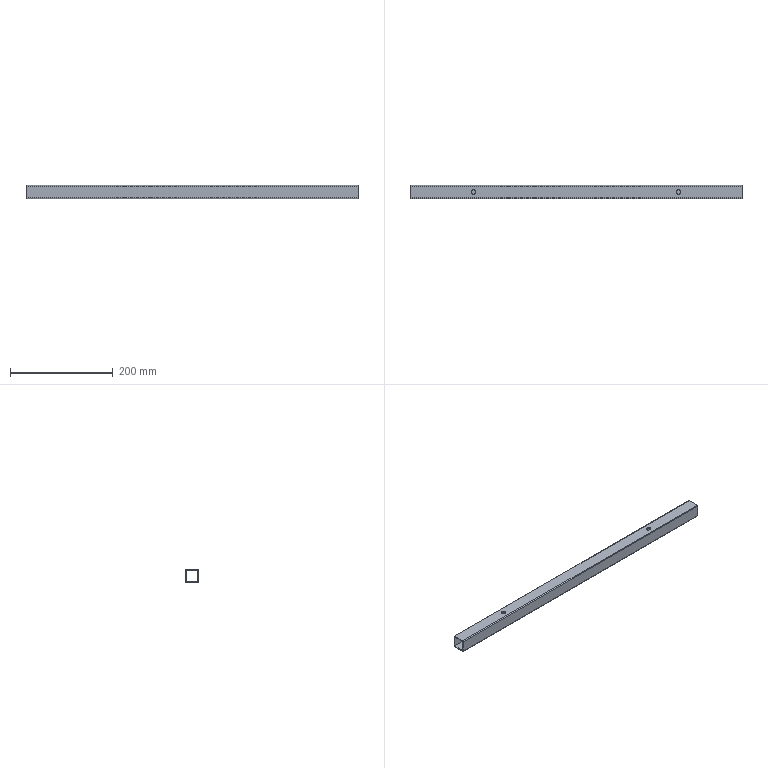Part | NX | features BREP 1 | 1 solid | 18 faces | box 647.7 x 25.4 x 25.4 mm | volume 112922 mm3 | plane 10 | cylinder 8 | commonest cylinder face diameters 3.175 x4 8.509 x4
STEP:
#1=CARTESIAN_POINT('',(-323.85,12.7,-11.113));
#2=VERTEX_POINT('',#1);
#3=CARTESIAN_POINT('',(-323.85,12.7,11.113));
#4=VERTEX_POINT('',#3);
#5=CARTESIAN_POINT('',(-323.85,12.7,-11.113));
#6=DIRECTION('',(0.,0.,1.));
#7=VECTOR('',#6,1000.);
#8=LINE('',#5,#7);
#9=EDGE_CURVE('',#2,#4,#8,.T.);
#10=ORIENTED_EDGE('',*,*,#9,.F.);
#11=CARTESIAN_POINT('',(-323.85,11.113,-12.7));
#12=VERTEX_POINT('',#11);
#13=CARTESIAN_POINT('',(-323.85,11.113,-11.113));
#14=DIRECTION('',(-1.,0.,0.));
#15=DIRECTION('',(0.,1.,0.));
#16=AXIS2_PLACEMENT_3D('',#13,#14,#15);
#17=CIRCLE('',#16,1.587);
#18=EDGE_CURVE('',#2,#12,#17,.T.);
#19=ORIENTED_EDGE('',*,*,#18,.T.);
#20=CARTESIAN_POINT('',(-323.85,-11.113,-12.7));
#21=VERTEX_POINT('',#20);
#22=CARTESIAN_POINT('',(-323.85,-11.113,-12.7));
#23=DIRECTION('',(0.,1.,0.));
#24=VECTOR('',#23,1000.);
#25=LINE('',#22,#24);
#26=EDGE_CURVE('',#21,#12,#25,.T.);
#27=ORIENTED_EDGE('',*,*,#26,.F.);
#28=CARTESIAN_POINT('',(-323.85,-12.7,-11.113));
#29=VERTEX_POINT('',#28);
#30=CARTESIAN_POINT('',(-323.85,-11.113,-11.113));
#31=DIRECTION('',(-1.,0.,0.));
#32=DIRECTION('',(0.,0.,-1.));
#33=AXIS2_PLACEMENT_3D('',#30,#31,#32);
#34=CIRCLE('',#33,1.587);
#35=EDGE_CURVE('',#21,#29,#34,.T.);
#36=ORIENTED_EDGE('',*,*,#35,.T.);
#37=CARTESIAN_POINT('',(-323.85,-12.7,11.113));
#38=VERTEX_POINT('',#37);
#39=CARTESIAN_POINT('',(-323.85,-12.7,11.113));
#40=DIRECTION('',(0.,0.,-1.));
#41=VECTOR('',#40,1000.);
#42=LINE('',#39,#41);
#43=EDGE_CURVE('',#38,#29,#42,.T.);
#44=ORIENTED_EDGE('',*,*,#43,.F.);
#45=CARTESIAN_POINT('',(-323.85,-11.113,12.7));
#46=VERTEX_POINT('',#45);
#47=CARTESIAN_POINT('',(-323.85,-11.113,11.113));
#48=DIRECTION('',(-1.,0.,0.));
#49=DIRECTION('',(0.,-1.,0.));
#50=AXIS2_PLACEMENT_3D('',#47,#48,#49);
#51=CIRCLE('',#50,1.587);
#52=EDGE_CURVE('',#38,#46,#51,.T.);
#53=ORIENTED_EDGE('',*,*,#52,.T.);
#54=CARTESIAN_POINT('',(-323.85,11.113,12.7));
#55=VERTEX_POINT('',#54);
#56=CARTESIAN_POINT('',(-323.85,11.113,12.7));
#57=DIRECTION('',(0.,-1.,0.));
#58=VECTOR('',#57,1000.);
#59=LINE('',#56,#58);
#60=EDGE_CURVE('',#55,#46,#59,.T.);
#61=ORIENTED_EDGE('',*,*,#60,.F.);
#62=CARTESIAN_POINT('',(-323.85,11.113,11.113));
#63=DIRECTION('',(-1.,0.,0.));
#64=DIRECTION('',(0.,0.,1.));
#65=AXIS2_PLACEMENT_3D('',#62,#63,#64);
#66=CIRCLE('',#65,1.587);
#67=EDGE_CURVE('',#55,#4,#66,.T.);
#68=ORIENTED_EDGE('',*,*,#67,.T.);
#69=EDGE_LOOP('',(#10,#19,#27,#36,#44,#53,#61,#68));
#70=FACE_BOUND('',#69,.T.);
#71=CARTESIAN_POINT('',(-323.85,10.82,10.82));
#72=VERTEX_POINT('',#71);
#73=CARTESIAN_POINT('',(-323.85,10.82,-10.82));
#74=VERTEX_POINT('',#73);
#75=CARTESIAN_POINT('',(-323.85,10.82,10.82));
#76=DIRECTION('',(0.,0.,-1.));
#77=VECTOR('',#76,1000.);
#78=LINE('',#75,#77);
#79=EDGE_CURVE('',#72,#74,#78,.T.);
#80=ORIENTED_EDGE('',*,*,#79,.F.);
#81=CARTESIAN_POINT('',(-323.85,-10.82,10.82));
#82=VERTEX_POINT('',#81);
#83=CARTESIAN_POINT('',(-323.85,-10.82,10.82));
#84=DIRECTION('',(0.,1.,0.));
#85=VECTOR('',#84,1000.);
#86=LINE('',#83,#85);
#87=EDGE_CURVE('',#82,#72,#86,.T.);
#88=ORIENTED_EDGE('',*,*,#87,.F.);
#89=CARTESIAN_POINT('',(-323.85,-10.82,-10.82));
#90=VERTEX_POINT('',#89);
#91=CARTESIAN_POINT('',(-323.85,-10.82,-10.82));
#92=DIRECTION('',(0.,0.,1.));
#93=VECTOR('',#92,1000.);
#94=LINE('',#91,#93);
#95=EDGE_CURVE('',#90,#82,#94,.T.);
#96=ORIENTED_EDGE('',*,*,#95,.F.);
#97=CARTESIAN_POINT('',(-323.85,10.82,-10.82));
#98=DIRECTION('',(0.,-1.,0.));
#99=VECTOR('',#98,1000.);
#100=LINE('',#97,#99);
#101=EDGE_CURVE('',#74,#90,#100,.T.);
#102=ORIENTED_EDGE('',*,*,#101,.F.);
#103=EDGE_LOOP('',(#80,#88,#96,#102));
#104=FACE_BOUND('',#103,.T.);
#105=CARTESIAN_POINT('',(-323.85,0.,0.));
#106=DIRECTION('',(1.,0.,0.));
#107=DIRECTION('',(0.,1.,0.));
#108=AXIS2_PLACEMENT_3D('',#105,#106,#107);
#109=PLANE('',#108);
#110=ADVANCED_FACE('',(#70,#104),#109,.F.);
#111=CARTESIAN_POINT('',(323.85,-10.82,-10.82));
#112=VERTEX_POINT('',#111);
#113=CARTESIAN_POINT('',(-323.85,-10.82,-10.82));
#114=DIRECTION('',(1.,0.,0.));
#115=VECTOR('',#114,1000.);
#116=LINE('',#113,#115);
#117=EDGE_CURVE('',#90,#112,#116,.T.);
#118=ORIENTED_EDGE('',*,*,#117,.T.);
#119=CARTESIAN_POINT('',(323.85,10.82,-10.82));
#120=VERTEX_POINT('',#119);
#121=CARTESIAN_POINT('',(323.85,10.82,-10.82));
#122=DIRECTION('',(0.,-1.,0.));
#123=VECTOR('',#122,1000.);
#124=LINE('',#121,#123);
#125=EDGE_CURVE('',#120,#112,#124,.T.);
#126=ORIENTED_EDGE('',*,*,#125,.F.);
#127=CARTESIAN_POINT('',(-323.85,10.82,-10.82));
#128=DIRECTION('',(1.,0.,0.));
#129=VECTOR('',#128,1000.);
#130=LINE('',#127,#129);
#131=EDGE_CURVE('',#74,#120,#130,.T.);
#132=ORIENTED_EDGE('',*,*,#131,.F.);
#133=ORIENTED_EDGE('',*,*,#101,.T.);
#134=EDGE_LOOP('',(#118,#126,#132,#133));
#135=FACE_BOUND('',#134,.T.);
#136=CARTESIAN_POINT('',(-323.85,10.82,-10.82));
#137=DIRECTION('',(0.,0.,1.));
#138=DIRECTION('',(1.,0.,0.));
#139=AXIS2_PLACEMENT_3D('',#136,#137,#138);
#140=PLANE('',#139);
#141=ADVANCED_FACE('',(#135),#140,.T.);
#142=ORIENTED_EDGE('',*,*,#131,.T.);
#143=CARTESIAN_POINT('',(323.85,10.82,10.82));
#144=VERTEX_POINT('',#143);
#145=CARTESIAN_POINT('',(323.85,10.82,10.82));
#146=DIRECTION('',(0.,0.,-1.));
#147=VECTOR('',#146,1000.);
#148=LINE('',#145,#147);
#149=EDGE_CURVE('',#144,#120,#148,.T.);
#150=ORIENTED_EDGE('',*,*,#149,.F.);
#151=CARTESIAN_POINT('',(-323.85,10.82,10.82));
#152=DIRECTION('',(1.,0.,0.));
#153=VECTOR('',#152,1000.);
#154=LINE('',#151,#153);
#155=EDGE_CURVE('',#72,#144,#154,.T.);
#156=ORIENTED_EDGE('',*,*,#155,.F.);
#157=ORIENTED_EDGE('',*,*,#79,.T.);
#158=EDGE_LOOP('',(#142,#150,#156,#157));
#159=FACE_BOUND('',#158,.T.);
#160=CARTESIAN_POINT('',(-323.85,10.82,10.82));
#161=DIRECTION('',(0.,-1.,0.));
#162=DIRECTION('',(0.,0.,-1.));
#163=AXIS2_PLACEMENT_3D('',#160,#161,#162);
#164=PLANE('',#163);
#165=ADVANCED_FACE('',(#159),#164,.T.);
#166=ORIENTED_EDGE('',*,*,#155,.T.);
#167=CARTESIAN_POINT('',(323.85,-10.82,10.82));
#168=VERTEX_POINT('',#167);
#169=CARTESIAN_POINT('',(323.85,-10.82,10.82));
#170=DIRECTION('',(0.,1.,0.));
#171=VECTOR('',#170,1000.);
#172=LINE('',#169,#171);
#173=EDGE_CURVE('',#168,#144,#172,.T.);
#174=ORIENTED_EDGE('',*,*,#173,.F.);
#175=CARTESIAN_POINT('',(-323.85,-10.82,10.82));
#176=DIRECTION('',(1.,0.,0.));
#177=VECTOR('',#176,1000.);
#178=LINE('',#175,#177);
#179=EDGE_CURVE('',#82,#168,#178,.T.);
#180=ORIENTED_EDGE('',*,*,#179,.F.);
#181=ORIENTED_EDGE('',*,*,#87,.T.);
#182=EDGE_LOOP('',(#166,#174,#180,#181));
#183=FACE_BOUND('',#182,.T.);
#184=CARTESIAN_POINT('',(204.28,0.,10.82));
#185=VERTEX_POINT('',#184);
#186=CARTESIAN_POINT('',(195.77,0.,10.82));
#187=VERTEX_POINT('',#186);
#188=CARTESIAN_POINT('',(200.025,0.,10.82));
#189=DIRECTION('',(0.,0.,-1.));
#190=DIRECTION('',(1.,0.,0.));
#191=AXIS2_PLACEMENT_3D('',#188,#189,#190);
#192=CIRCLE('',#191,4.254);
#193=EDGE_CURVE('',#185,#187,#192,.T.);
#194=ORIENTED_EDGE('',*,*,#193,.F.);
#195=CARTESIAN_POINT('',(200.025,0.,10.82));
#196=DIRECTION('',(0.,0.,-1.));
#197=DIRECTION('',(-1.,0.,0.));
#198=AXIS2_PLACEMENT_3D('',#195,#196,#197);
#199=CIRCLE('',#198,4.254);
#200=EDGE_CURVE('',#187,#185,#199,.T.);
#201=ORIENTED_EDGE('',*,*,#200,.F.);
#202=EDGE_LOOP('',(#194,#201));
#203=FACE_BOUND('',#202,.T.);
#204=CARTESIAN_POINT('',(-204.28,0.,10.82));
#205=VERTEX_POINT('',#204);
#206=CARTESIAN_POINT('',(-195.77,0.,10.82));
#207=VERTEX_POINT('',#206);
#208=CARTESIAN_POINT('',(-200.025,0.,10.82));
#209=DIRECTION('',(0.,0.,1.));
#210=DIRECTION('',(-1.,0.,0.));
#211=AXIS2_PLACEMENT_3D('',#208,#209,#210);
#212=CIRCLE('',#211,4.254);
#213=EDGE_CURVE('',#205,#207,#212,.T.);
#214=ORIENTED_EDGE('',*,*,#213,.T.);
#215=CARTESIAN_POINT('',(-200.025,0.,10.82));
#216=DIRECTION('',(0.,0.,1.));
#217=DIRECTION('',(1.,0.,0.));
#218=AXIS2_PLACEMENT_3D('',#215,#216,#217);
#219=CIRCLE('',#218,4.254);
#220=EDGE_CURVE('',#207,#205,#219,.T.);
#221=ORIENTED_EDGE('',*,*,#220,.T.);
#222=EDGE_LOOP('',(#214,#221));
#223=FACE_BOUND('',#222,.T.);
#224=CARTESIAN_POINT('',(-323.85,-10.82,10.82));
#225=DIRECTION('',(0.,0.,-1.));
#226=DIRECTION('',(0.,-1.,0.));
#227=AXIS2_PLACEMENT_3D('',#224,#225,#226);
#228=PLANE('',#227);
#229=ADVANCED_FACE('',(#183,#203,#223),#228,.T.);
#230=ORIENTED_EDGE('',*,*,#179,.T.);
#231=CARTESIAN_POINT('',(323.85,-10.82,-10.82));
#232=DIRECTION('',(0.,0.,1.));
#233=VECTOR('',#232,1000.);
#234=LINE('',#231,#233);
#235=EDGE_CURVE('',#112,#168,#234,.T.);
#236=ORIENTED_EDGE('',*,*,#235,.F.);
#237=ORIENTED_EDGE('',*,*,#117,.F.);
#238=ORIENTED_EDGE('',*,*,#95,.T.);
#239=EDGE_LOOP('',(#230,#236,#237,#238));
#240=FACE_BOUND('',#239,.T.);
#241=CARTESIAN_POINT('',(-323.85,-10.82,-10.82));
#242=DIRECTION('',(0.,1.,0.));
#243=DIRECTION('',(1.,0.,0.));
#244=AXIS2_PLACEMENT_3D('',#241,#242,#243);
#245=PLANE('',#244);
#246=ADVANCED_FACE('',(#240),#245,.T.);
#247=CARTESIAN_POINT('',(323.85,11.113,12.7));
#248=VERTEX_POINT('',#247);
#249=CARTESIAN_POINT('',(323.85,-11.113,12.7));
#250=VERTEX_POINT('',#249);
#251=CARTESIAN_POINT('',(323.85,11.113,12.7));
#252=DIRECTION('',(0.,-1.,0.));
#253=VECTOR('',#252,1000.);
#254=LINE('',#251,#253);
#255=EDGE_CURVE('',#248,#250,#254,.T.);
#256=ORIENTED_EDGE('',*,*,#255,.T.);
#257=CARTESIAN_POINT('',(323.85,-12.7,11.113));
#258=VERTEX_POINT('',#257);
#259=CARTESIAN_POINT('',(323.85,-11.113,11.113));
#260=DIRECTION('',(1.,0.,0.));
#261=DIRECTION('',(0.,0.,1.));
#262=AXIS2_PLACEMENT_3D('',#259,#260,#261);
#263=CIRCLE('',#262,1.587);
#264=EDGE_CURVE('',#250,#258,#263,.T.);
#265=ORIENTED_EDGE('',*,*,#264,.T.);
#266=CARTESIAN_POINT('',(323.85,-12.7,-11.113));
#267=VERTEX_POINT('',#266);
#268=CARTESIAN_POINT('',(323.85,-12.7,11.113));
#269=DIRECTION('',(0.,0.,-1.));
#270=VECTOR('',#269,1000.);
#271=LINE('',#268,#270);
#272=EDGE_CURVE('',#258,#267,#271,.T.);
#273=ORIENTED_EDGE('',*,*,#272,.T.);
#274=CARTESIAN_POINT('',(323.85,-11.113,-12.7));
#275=VERTEX_POINT('',#274);
#276=CARTESIAN_POINT('',(323.85,-11.113,-11.113));
#277=DIRECTION('',(1.,0.,0.));
#278=DIRECTION('',(0.,-1.,0.));
#279=AXIS2_PLACEMENT_3D('',#276,#277,#278);
#280=CIRCLE('',#279,1.587);
#281=EDGE_CURVE('',#267,#275,#280,.T.);
#282=ORIENTED_EDGE('',*,*,#281,.T.);
#283=CARTESIAN_POINT('',(323.85,11.113,-12.7));
#284=VERTEX_POINT('',#283);
#285=CARTESIAN_POINT('',(323.85,-11.113,-12.7));
#286=DIRECTION('',(0.,1.,0.));
#287=VECTOR('',#286,1000.);
#288=LINE('',#285,#287);
#289=EDGE_CURVE('',#275,#284,#288,.T.);
#290=ORIENTED_EDGE('',*,*,#289,.T.);
#291=CARTESIAN_POINT('',(323.85,12.7,-11.113));
#292=VERTEX_POINT('',#291);
#293=CARTESIAN_POINT('',(323.85,11.113,-11.113));
#294=DIRECTION('',(1.,0.,0.));
#295=DIRECTION('',(0.,0.,-1.));
#296=AXIS2_PLACEMENT_3D('',#293,#294,#295);
#297=CIRCLE('',#296,1.587);
#298=EDGE_CURVE('',#284,#292,#297,.T.);
#299=ORIENTED_EDGE('',*,*,#298,.T.);
#300=CARTESIAN_POINT('',(323.85,12.7,11.113));
#301=VERTEX_POINT('',#300);
#302=CARTESIAN_POINT('',(323.85,12.7,-11.113));
#303=DIRECTION('',(0.,0.,1.));
#304=VECTOR('',#303,1000.);
#305=LINE('',#302,#304);
#306=EDGE_CURVE('',#292,#301,#305,.T.);
#307=ORIENTED_EDGE('',*,*,#306,.T.);
#308=CARTESIAN_POINT('',(323.85,11.113,11.113));
#309=DIRECTION('',(1.,0.,0.));
#310=DIRECTION('',(0.,1.,0.));
#311=AXIS2_PLACEMENT_3D('',#308,#309,#310);
#312=CIRCLE('',#311,1.587);
#313=EDGE_CURVE('',#301,#248,#312,.T.);
#314=ORIENTED_EDGE('',*,*,#313,.T.);
#315=EDGE_LOOP('',(#256,#265,#273,#282,#290,#299,#307,#314));
#316=FACE_BOUND('',#315,.T.);
#317=ORIENTED_EDGE('',*,*,#235,.T.);
#318=ORIENTED_EDGE('',*,*,#173,.T.);
#319=ORIENTED_EDGE('',*,*,#149,.T.);
#320=ORIENTED_EDGE('',*,*,#125,.T.);
#321=EDGE_LOOP('',(#317,#318,#319,#320));
#322=FACE_BOUND('',#321,.T.);
#323=CARTESIAN_POINT('',(323.85,0.,0.));
#324=DIRECTION('',(1.,0.,0.));
#325=DIRECTION('',(0.,1.,0.));
#326=AXIS2_PLACEMENT_3D('',#323,#324,#325);
#327=PLANE('',#326);
#328=ADVANCED_FACE('',(#316,#322),#327,.T.);
#329=ORIENTED_EDGE('',*,*,#313,.F.);
#330=CARTESIAN_POINT('',(323.85,12.7,11.113));
#331=DIRECTION('',(-1.,0.,0.));
#332=VECTOR('',#331,1000.);
#333=LINE('',#330,#332);
#334=EDGE_CURVE('',#301,#4,#333,.T.);
#335=ORIENTED_EDGE('',*,*,#334,.T.);
#336=ORIENTED_EDGE('',*,*,#67,.F.);
#337=CARTESIAN_POINT('',(323.85,11.113,12.7));
#338=DIRECTION('',(-1.,0.,0.));
#339=VECTOR('',#338,1000.);
#340=LINE('',#337,#339);
#341=EDGE_CURVE('',#248,#55,#340,.T.);
#342=ORIENTED_EDGE('',*,*,#341,.F.);
#343=EDGE_LOOP('',(#329,#335,#336,#342));
#344=FACE_BOUND('',#343,.T.);
#345=CARTESIAN_POINT('',(324.865,11.113,11.113));
#346=DIRECTION('',(-1.,0.,0.));
#347=DIRECTION('',(0.,0.,1.));
#348=AXIS2_PLACEMENT_3D('',#345,#346,#347);
#349=CYLINDRICAL_SURFACE('',#348,1.587);
#350=ADVANCED_FACE('',(#344),#349,.T.);
#351=ORIENTED_EDGE('',*,*,#60,.T.);
#352=CARTESIAN_POINT('',(323.85,-11.113,12.7));
#353=DIRECTION('',(-1.,0.,0.));
#354=VECTOR('',#353,1000.);
#355=LINE('',#352,#354);
#356=EDGE_CURVE('',#250,#46,#355,.T.);
#357=ORIENTED_EDGE('',*,*,#356,.F.);
#358=ORIENTED_EDGE('',*,*,#255,.F.);
#359=ORIENTED_EDGE('',*,*,#341,.T.);
#360=EDGE_LOOP('',(#351,#357,#358,#359));
#361=FACE_BOUND('',#360,.T.);
#362=CARTESIAN_POINT('',(204.28,0.,12.7));
#363=VERTEX_POINT('',#362);
#364=CARTESIAN_POINT('',(195.77,0.,12.7));
#365=VERTEX_POINT('',#364);
#366=CARTESIAN_POINT('',(200.025,0.,12.7));
#367=DIRECTION('',(0.,0.,-1.));
#368=DIRECTION('',(1.,0.,0.));
#369=AXIS2_PLACEMENT_3D('',#366,#367,#368);
#370=CIRCLE('',#369,4.254);
#371=EDGE_CURVE('',#363,#365,#370,.T.);
#372=ORIENTED_EDGE('',*,*,#371,.T.);
#373=CARTESIAN_POINT('',(200.025,0.,12.7));
#374=DIRECTION('',(0.,0.,-1.));
#375=DIRECTION('',(-1.,0.,0.));
#376=AXIS2_PLACEMENT_3D('',#373,#374,#375);
#377=CIRCLE('',#376,4.254);
#378=EDGE_CURVE('',#365,#363,#377,.T.);
#379=ORIENTED_EDGE('',*,*,#378,.T.);
#380=EDGE_LOOP('',(#372,#379));
#381=FACE_BOUND('',#380,.T.);
#382=CARTESIAN_POINT('',(-204.28,0.,12.7));
#383=VERTEX_POINT('',#382);
#384=CARTESIAN_POINT('',(-195.77,0.,12.7));
#385=VERTEX_POINT('',#384);
#386=CARTESIAN_POINT('',(-200.025,0.,12.7));
#387=DIRECTION('',(0.,0.,1.));
#388=DIRECTION('',(-1.,0.,0.));
#389=AXIS2_PLACEMENT_3D('',#386,#387,#388);
#390=CIRCLE('',#389,4.254);
#391=EDGE_CURVE('',#383,#385,#390,.T.);
#392=ORIENTED_EDGE('',*,*,#391,.F.);
#393=CARTESIAN_POINT('',(-200.025,0.,12.7));
#394=DIRECTION('',(0.,0.,1.));
#395=DIRECTION('',(1.,0.,0.));
#396=AXIS2_PLACEMENT_3D('',#393,#394,#395);
#397=CIRCLE('',#396,4.254);
#398=EDGE_CURVE('',#385,#383,#397,.T.);
#399=ORIENTED_EDGE('',*,*,#398,.F.);
#400=EDGE_LOOP('',(#392,#399));
#401=FACE_BOUND('',#400,.T.);
#402=CARTESIAN_POINT('',(-323.85,12.7,12.7));
#403=DIRECTION('',(0.,0.,1.));
#404=DIRECTION('',(1.,0.,0.));
#405=AXIS2_PLACEMENT_3D('',#402,#403,#404);
#406=PLANE('',#405);
#407=ADVANCED_FACE('',(#361,#381,#401),#406,.T.);
#408=ORIENTED_EDGE('',*,*,#264,.F.);
#409=ORIENTED_EDGE('',*,*,#356,.T.);
#410=ORIENTED_EDGE('',*,*,#52,.F.);
#411=CARTESIAN_POINT('',(323.85,-12.7,11.113));
#412=DIRECTION('',(-1.,0.,0.));
#413=VECTOR('',#412,1000.);
#414=LINE('',#411,#413);
#415=EDGE_CURVE('',#258,#38,#414,.T.);
#416=ORIENTED_EDGE('',*,*,#415,.F.);
#417=EDGE_LOOP('',(#408,#409,#410,#416));
#418=FACE_BOUND('',#417,.T.);
#419=CARTESIAN_POINT('',(324.865,-11.113,11.113));
#420=DIRECTION('',(-1.,0.,0.));
#421=DIRECTION('',(0.,-1.,0.));
#422=AXIS2_PLACEMENT_3D('',#419,#420,#421);
#423=CYLINDRICAL_SURFACE('',#422,1.587);
#424=ADVANCED_FACE('',(#418),#423,.T.);
#425=ORIENTED_EDGE('',*,*,#43,.T.);
#426=CARTESIAN_POINT('',(323.85,-12.7,-11.113));
#427=DIRECTION('',(-1.,0.,0.));
#428=VECTOR('',#427,1000.);
#429=LINE('',#426,#428);
#430=EDGE_CURVE('',#267,#29,#429,.T.);
#431=ORIENTED_EDGE('',*,*,#430,.F.);
#432=ORIENTED_EDGE('',*,*,#272,.F.);
#433=ORIENTED_EDGE('',*,*,#415,.T.);
#434=EDGE_LOOP('',(#425,#431,#432,#433));
#435=FACE_BOUND('',#434,.T.);
#436=CARTESIAN_POINT('',(-323.85,-12.7,12.7));
#437=DIRECTION('',(0.,-1.,0.));
#438=DIRECTION('',(0.,0.,-1.));
#439=AXIS2_PLACEMENT_3D('',#436,#437,#438);
#440=PLANE('',#439);
#441=ADVANCED_FACE('',(#435),#440,.T.);
#442=ORIENTED_EDGE('',*,*,#281,.F.);
#443=ORIENTED_EDGE('',*,*,#430,.T.);
#444=ORIENTED_EDGE('',*,*,#35,.F.);
#445=CARTESIAN_POINT('',(323.85,-11.113,-12.7));
#446=DIRECTION('',(-1.,0.,0.));
#447=VECTOR('',#446,1000.);
#448=LINE('',#445,#447);
#449=EDGE_CURVE('',#275,#21,#448,.T.);
#450=ORIENTED_EDGE('',*,*,#449,.F.);
#451=EDGE_LOOP('',(#442,#443,#444,#450));
#452=FACE_BOUND('',#451,.T.);
#453=CARTESIAN_POINT('',(324.865,-11.113,-11.113));
#454=DIRECTION('',(-1.,0.,0.));
#455=DIRECTION('',(0.,0.,-1.));
#456=AXIS2_PLACEMENT_3D('',#453,#454,#455);
#457=CYLINDRICAL_SURFACE('',#456,1.587);
#458=ADVANCED_FACE('',(#452),#457,.T.);
#459=ORIENTED_EDGE('',*,*,#289,.F.);
#460=ORIENTED_EDGE('',*,*,#449,.T.);
#461=ORIENTED_EDGE('',*,*,#26,.T.);
#462=CARTESIAN_POINT('',(323.85,11.113,-12.7));
#463=DIRECTION('',(-1.,0.,0.));
#464=VECTOR('',#463,1000.);
#465=LINE('',#462,#464);
#466=EDGE_CURVE('',#284,#12,#465,.T.);
#467=ORIENTED_EDGE('',*,*,#466,.F.);
#468=EDGE_LOOP('',(#459,#460,#461,#467));
#469=FACE_BOUND('',#468,.T.);
#470=CARTESIAN_POINT('',(-323.85,-12.7,-12.7));
#471=DIRECTION('',(0.,0.,-1.));
#472=DIRECTION('',(0.,-1.,0.));
#473=AXIS2_PLACEMENT_3D('',#470,#471,#472);
#474=PLANE('',#473);
#475=ADVANCED_FACE('',(#469),#474,.T.);
#476=ORIENTED_EDGE('',*,*,#298,.F.);
#477=ORIENTED_EDGE('',*,*,#466,.T.);
#478=ORIENTED_EDGE('',*,*,#18,.F.);
#479=CARTESIAN_POINT('',(323.85,12.7,-11.113));
#480=DIRECTION('',(-1.,0.,0.));
#481=VECTOR('',#480,1000.);
#482=LINE('',#479,#481);
#483=EDGE_CURVE('',#292,#2,#482,.T.);
#484=ORIENTED_EDGE('',*,*,#483,.F.);
#485=EDGE_LOOP('',(#476,#477,#478,#484));
#486=FACE_BOUND('',#485,.T.);
#487=CARTESIAN_POINT('',(324.865,11.113,-11.113));
#488=DIRECTION('',(-1.,0.,0.));
#489=DIRECTION('',(0.,1.,0.));
#490=AXIS2_PLACEMENT_3D('',#487,#488,#489);
#491=CYLINDRICAL_SURFACE('',#490,1.587);
#492=ADVANCED_FACE('',(#486),#491,.T.);
#493=ORIENTED_EDGE('',*,*,#306,.F.);
#494=ORIENTED_EDGE('',*,*,#483,.T.);
#495=ORIENTED_EDGE('',*,*,#9,.T.);
#496=ORIENTED_EDGE('',*,*,#334,.F.);
#497=EDGE_LOOP('',(#493,#494,#495,#496));
#498=FACE_BOUND('',#497,.T.);
#499=CARTESIAN_POINT('',(-323.85,12.7,-12.7));
#500=DIRECTION('',(0.,1.,0.));
#501=DIRECTION('',(1.,0.,0.));
#502=AXIS2_PLACEMENT_3D('',#499,#500,#501);
#503=PLANE('',#502);
#504=ADVANCED_FACE('',(#498),#503,.T.);
#505=CARTESIAN_POINT('',(195.77,0.,12.7));
#506=DIRECTION('',(0.,0.,-1.));
#507=VECTOR('',#506,1000.);
#508=LINE('',#505,#507);
#509=EDGE_CURVE('',#365,#187,#508,.T.);
#510=ORIENTED_EDGE('',*,*,#509,.T.);
#511=ORIENTED_EDGE('',*,*,#200,.T.);
#512=CARTESIAN_POINT('',(204.28,0.,12.7));
#513=DIRECTION('',(0.,0.,-1.));
#514=VECTOR('',#513,1000.);
#515=LINE('',#512,#514);
#516=EDGE_CURVE('',#363,#185,#515,.T.);
#517=ORIENTED_EDGE('',*,*,#516,.F.);
#518=ORIENTED_EDGE('',*,*,#378,.F.);
#519=EDGE_LOOP('',(#510,#511,#517,#518));
#520=FACE_BOUND('',#519,.T.);
#521=CARTESIAN_POINT('',(200.025,0.,12.7));
#522=DIRECTION('',(0.,0.,-1.));
#523=DIRECTION('',(-1.,0.,0.));
#524=AXIS2_PLACEMENT_3D('',#521,#522,#523);
#525=CYLINDRICAL_SURFACE('',#524,4.254);
#526=ADVANCED_FACE('',(#520),#525,.F.);
#527=ORIENTED_EDGE('',*,*,#516,.T.);
#528=ORIENTED_EDGE('',*,*,#193,.T.);
#529=ORIENTED_EDGE('',*,*,#509,.F.);
#530=ORIENTED_EDGE('',*,*,#371,.F.);
#531=EDGE_LOOP('',(#527,#528,#529,#530));
#532=FACE_BOUND('',#531,.T.);
#533=CARTESIAN_POINT('',(200.025,0.,12.7));
#534=DIRECTION('',(0.,0.,-1.));
#535=DIRECTION('',(-1.,0.,0.));
#536=AXIS2_PLACEMENT_3D('',#533,#534,#535);
#537=CYLINDRICAL_SURFACE('',#536,4.254);
#538=ADVANCED_FACE('',(#532),#537,.F.);
#539=CARTESIAN_POINT('',(-204.28,0.,12.7));
#540=DIRECTION('',(0.,0.,-1.));
#541=VECTOR('',#540,1000.);
#542=LINE('',#539,#541);
#543=EDGE_CURVE('',#383,#205,#542,.T.);
#544=ORIENTED_EDGE('',*,*,#543,.T.);
#545=ORIENTED_EDGE('',*,*,#220,.F.);
#546=CARTESIAN_POINT('',(-195.77,0.,12.7));
#547=DIRECTION('',(0.,0.,-1.));
#548=VECTOR('',#547,1000.);
#549=LINE('',#546,#548);
#550=EDGE_CURVE('',#385,#207,#549,.T.);
#551=ORIENTED_EDGE('',*,*,#550,.F.);
#552=ORIENTED_EDGE('',*,*,#398,.T.);
#553=EDGE_LOOP('',(#544,#545,#551,#552));
#554=FACE_BOUND('',#553,.T.);
#555=CARTESIAN_POINT('',(-200.025,0.,12.7));
#556=DIRECTION('',(0.,0.,1.));
#557=DIRECTION('',(1.,0.,0.));
#558=AXIS2_PLACEMENT_3D('',#555,#556,#557);
#559=CYLINDRICAL_SURFACE('',#558,4.254);
#560=ADVANCED_FACE('',(#554),#559,.F.);
#561=ORIENTED_EDGE('',*,*,#550,.T.);
#562=ORIENTED_EDGE('',*,*,#213,.F.);
#563=ORIENTED_EDGE('',*,*,#543,.F.);
#564=ORIENTED_EDGE('',*,*,#391,.T.);
#565=EDGE_LOOP('',(#561,#562,#563,#564));
#566=FACE_BOUND('',#565,.T.);
#567=CARTESIAN_POINT('',(-200.025,0.,12.7));
#568=DIRECTION('',(0.,0.,1.));
#569=DIRECTION('',(1.,0.,0.));
#570=AXIS2_PLACEMENT_3D('',#567,#568,#569);
#571=CYLINDRICAL_SURFACE('',#570,4.254);
#572=ADVANCED_FACE('',(#566),#571,.F.);
#573=CLOSED_SHELL('',(#110,#141,#165,#229,#246,#328,#350,#407,#424,#441,#458,#475,#492,#504,#526,#538,#560,#572));
#574=MANIFOLD_SOLID_BREP('',#573);
#575=(LENGTH_UNIT()NAMED_UNIT(*)SI_UNIT(.MILLI.,.METRE.));
#576=UNCERTAINTY_MEASURE_WITH_UNIT(LENGTH_MEASURE(0.00001),#575,'','');
#577=(NAMED_UNIT(*)PLANE_ANGLE_UNIT()SI_UNIT($,.RADIAN.));
#578=(NAMED_UNIT(*)SI_UNIT($,.STERADIAN.)SOLID_ANGLE_UNIT());
#579=(GEOMETRIC_REPRESENTATION_CONTEXT(3)GLOBAL_UNCERTAINTY_ASSIGNED_CONTEXT((#576))GLOBAL_UNIT_ASSIGNED_CONTEXT((#575,#577,#578))REPRESENTATION_CONTEXT('',''));
#580=ADVANCED_BREP_SHAPE_REPRESENTATION('',(#574),#579);